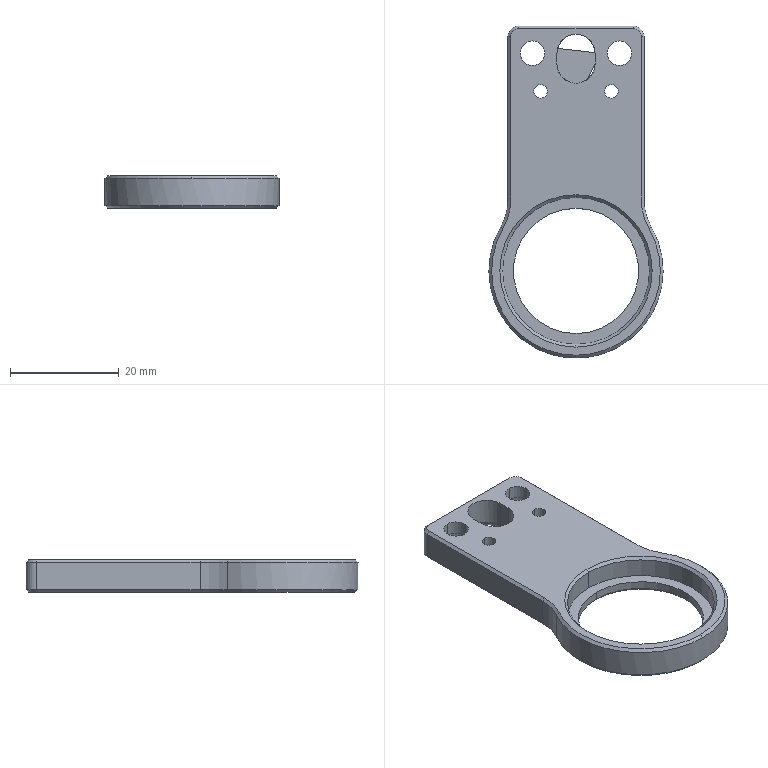NC program | NX | posted with a generic post | part box 32 x 61 x 6 mm
Lines 1418 to 2395 of 12533:
(ZLEVEL_PROFILE_1 , TOOL : D3R0.5)
N2816 T18 M6
N2818 G54
N2820 G17 G0 G90 X-13.711 Y2.712 S9500 M3
N2822 G43 Z30. H18
N2824 Z1.488
N2826 G94 G1 Z-0.012 F1000.
N2828 X-13.97 Y3.162
N2830 G3 X-14.23 Y3.312 R0.3
N2832 G1 X-23.46 F2500.
N2834 G3 X-25.864 Y2.367 R3.526
N2836 X-26.227 Y1.5 R1.142
N2838 G1 Y-1.5
N2840 G3 X-25.467 Y-2.711 R1.707
N2842 X-23.445 Y-3.312 R3.7
N2844 G1 X-5.
N2846 G3 X-1.688 Y0. R3.312
N2848 X-5. Y3.312 R3.312
N2850 G1 X-14.23
N2852 X-15.384 Y3.31
N2854 X-16.538 Y3.307
N2856 X-17.691 Y3.304 Z-0.013
N2858 X-18.845 Y3.302
N2860 X-19.999 Y3.299 Z-0.014
N2862 X-21.153 Y3.296
N2864 X-22.28 Y3.294
N2866 X-23.46 Y3.295 Z-0.015
N2868 X-23.98 Y3.228
N2870 X-24.486 Y3.104
N2872 X-24.977 Y2.928
N2874 X-25.437 Y2.676
N2876 X-25.832 Y2.346
N2878 X-25.989 Y2.165
N2880 X-26.107 Y1.954 Z-0.016
N2882 X-26.186 Y1.728
N2884 X-26.205 Y1.629
N2886 X-26.203 Y1.5
N2888 X-26.196 Y0.75
N2890 X-26.195 Y0.
N2892 X-26.193 Y-0.75
N2894 X-26.192 Y-1.5 Z-0.017
N2896 X-26.182 Y-1.682
N2898 X-26.11 Y-1.845
N2900 X-26.032 Y-2.008
N2902 X-25.947 Y-2.167
N2904 X-25.843 Y-2.3
N2906 X-25.713 Y-2.439
N2908 X-25.503 Y-2.604
N2910 X-25.428 Y-2.656
N2912 X-25.201 Y-2.793
N2914 X-24.97 Y-2.91
N2916 X-24.728 Y-3.014
N2918 X-24.48 Y-3.098
N2920 X-24.226 Y-3.165
N2922 X-23.969 Y-3.215 Z-0.018
N2924 X-23.486 Y-3.265
N2926 X-23.445 Y-3.267
N2928 X-22.127 Y-3.268
N2930 X-20.81 Y-3.265 Z-0.019
N2932 X-19.492 Y-3.263
N2934 X-18.175 Y-3.26
N2936 X-16.857 Y-3.258 Z-0.02
N2938 X-15.54 Y-3.255
N2940 X-14.222 Y-3.253 Z-0.021
N2942 X-12.905 Y-3.25
N2944 X-11.587 Y-3.248
N2946 X-10.27 Y-3.246 Z-0.022
N2948 X-8.952 Y-3.243
N2950 X-7.635 Y-3.241 Z-0.023
N2952 X-6.317 Y-3.239
N2954 X-5. Y-3.236
N2956 X-4.769 Y-3.228
N2958 X-4.54 Y-3.203
N2960 X-4.313 Y-3.161 Z-0.024
N2962 X-4.089 Y-3.104
N2964 X-3.87 Y-3.031
N2966 X-3.657 Y-2.942
N2968 X-3.451 Y-2.839
N2970 X-3.253 Y-2.721
N2972 X-3.064 Y-2.589
N2974 X-2.884 Y-2.444
N2976 X-2.716 Y-2.287
N2978 X-2.559 Y-2.118
N2980 X-2.415 Y-1.938
N2982 X-2.283 Y-1.749
N2984 X-2.166 Y-1.55
N2986 X-2.063 Y-1.344
N2988 X-1.975 Y-1.131 Z-0.025
N2990 X-1.902 Y-0.913
N2992 X-1.845 Y-0.69
N2994 X-1.805 Y-0.463
N2996 X-1.78 Y-0.234
N2998 X-1.772 Y-0.004
N3000 X-1.781 Y0.227
N3002 X-1.805 Y0.456
N3004 X-1.846 Y0.683
N3006 X-1.904 Y0.906
N3008 X-1.976 Y1.125
N3010 X-2.065 Y1.337
N3012 X-2.168 Y1.543
N3014 X-2.286 Y1.741
N3016 X-2.417 Y1.931 Z-0.026
N3018 X-2.562 Y2.11
N3020 X-2.719 Y2.278
N3022 X-2.888 Y2.435
N3024 X-3.067 Y2.579
N3026 X-3.257 Y2.71
N3028 X-3.455 Y2.827
N3030 X-3.661 Y2.93
N3032 X-3.873 Y3.018
N3034 X-4.092 Y3.09
N3036 X-4.315 Y3.147
N3038 X-4.541 Y3.187
N3040 X-4.77 Y3.212
N3042 X-5. Y3.22
N3044 X-6.154 Y3.218 Z-0.027
N3046 X-7.308 Y3.216
N3048 X-8.461 Y3.214 Z-0.028
N3050 X-9.615 Y3.212
N3052 X-10.769 Y3.21
N3054 X-11.923 Y3.209 Z-0.029
N3056 X-13.076 Y3.207
N3058 X-14.23 Y3.205
N3060 X-15.377 Y3.203 Z-0.03
N3062 X-16.524 Y3.2
N3064 X-17.671 Y3.198 Z-0.031
N3066 X-18.818 Y3.196
N3068 X-19.965 Y3.193 Z-0.032
N3070 X-21.112 Y3.191
N3072 X-22.259 Y3.189 Z-0.033
N3074 X-23.406
N3076 X-23.917 Y3.15
N3078 X-24.417 Y3.035 Z-0.034
N3080 X-24.895 Y2.851
N3082 X-25.34 Y2.597
N3084 X-25.629 Y2.379
N3086 X-25.735 Y2.276
N3088 X-25.89 Y2.073
N3090 X-26.012 Y1.869
N3092 X-26.108 Y1.618
N3094 X-26.097 Y1.5 Z-0.035
N3096 X-26.093 Y0.75
N3098 X-26.091 Y0.
N3100 X-26.09 Y-0.75
N3102 X-26.088 Y-1.5 Z-0.036
N3104 X-26.082 Y-1.666
N3106 X-26.02 Y-1.799
N3108 X-25.953 Y-1.94
N3110 X-25.876 Y-2.078
N3112 X-25.787 Y-2.195
N3114 X-25.677 Y-2.317
N3116 X-25.424 Y-2.533
N3118 X-25.087 Y-2.742
N3120 X-24.708 Y-2.918 Z-0.037
N3122 X-24.308 Y-3.041
N3124 X-23.9 Y-3.125
N3126 X-23.484 Y-3.171
N3128 X-23.348
N3130 X-22.096 Y-3.166 Z-0.038
N3132 X-20.844 Y-3.163
N3134 X-19.524 Y-3.161 Z-0.039
N3136 X-18.204 Y-3.158
N3138 X-16.883 Y-3.156 Z-0.04
N3140 X-15.563 Y-3.154
N3142 X-14.243 Y-3.151 Z-0.041
N3144 X-12.922 Y-3.149 Z-0.042
N3146 X-11.602 Y-3.147
N3148 X-10.281 Y-3.145 Z-0.043
N3150 X-8.961 Y-3.142
N3152 X-7.641 Y-3.14 Z-0.044
N3154 X-6.32 Y-3.138
N3156 X-5. Y-3.136 Z-0.045
N3158 X-4.754 Y-3.126
N3160 X-4.51 Y-3.096
N3162 X-4.269 Y-3.048
N3164 X-4.033 Y-2.981
N3166 X-3.802 Y-2.896
N3168 X-3.579 Y-2.792 Z-0.046
N3170 X-3.365 Y-2.672
N3172 X-3.161 Y-2.535
N3174 X-2.968 Y-2.383
N3176 X-2.787 Y-2.216
N3178 X-2.621 Y-2.036
N3180 X-2.469 Y-1.843
N3182 X-2.333 Y-1.639
N3184 X-2.213 Y-1.424
N3186 X-2.11 Y-1.201
N3188 X-2.025 Y-0.971 Z-0.047
N3190 X-1.959 Y-0.735
N3192 X-1.911 Y-0.494
N3194 X-1.882 Y-0.25
N3196 X-1.872 Y-0.005
N3198 X-1.882 Y0.24
N3200 X-1.911 Y0.484
N3202 X-1.959 Y0.725
N3204 X-2.026 Y0.962
N3206 X-2.111 Y1.192
N3208 X-2.214 Y1.416 Z-0.048
N3210 X-2.334 Y1.63
N3212 X-2.47 Y1.834
N3214 X-2.623 Y2.027
N3216 X-2.789 Y2.207
N3218 X-2.97 Y2.373
N3220 X-3.163 Y2.525
N3222 X-3.367 Y2.661
N3224 X-3.581 Y2.781
N3226 X-3.804 Y2.884 Z-0.049
N3228 X-4.034 Y2.968
N3230 X-4.271 Y3.034
N3232 X-4.511 Y3.082
N3234 X-4.755 Y3.11
N3236 X-5. Y3.12
N3238 X-6.154 Y3.118
N3240 X-7.308 Y3.116 Z-0.05
N3242 X-8.461 Y3.114
N3244 X-9.615 Y3.112 Z-0.051
N3246 X-10.769 Y3.111
N3248 X-11.923 Y3.109 Z-0.052
N3250 X-13.076 Y3.107
N3252 X-14.23 Y3.105 Z-0.053
N3254 X-15.374 Y3.103
N3256 X-16.519 Y3.101 Z-0.054
N3258 X-17.663 Y3.099 Z-0.055
N3260 X-18.807 Y3.096
N3262 X-19.952 Y3.094 Z-0.056
N3264 X-21.096 Y3.092 Z-0.057
N3266 X-22.206 Y3.09
N3268 X-23.315 Y3.089 Z-0.058
N3270 X-23.384
N3272 X-23.855 Y3.049
N3274 X-24.315 Y2.945
N3276 X-24.764 Y2.797 Z-0.059
N3278 X-25.183 Y2.579
N3280 X-25.487 Y2.372
N3282 X-25.568 Y2.307
N3284 X-25.73 Y2.137
N3286 X-25.809 Y2.026
N3288 X-25.863 Y1.944
N3290 X-25.899 Y1.876
N3292 X-25.917 Y1.842
N3294 X-25.933 Y1.806
N3296 X-25.952 Y1.728
N3298 X-25.999 Y1.5 Z-0.06
N3300 X-25.994 Y0.75
N3302 X-25.993 Y0.
N3304 X-25.992 Y-0.75 Z-0.061
N3306 X-25.993 Y-1.5
N3308 X-25.985 Y-1.591
N3310 X-25.968 Y-1.687
N3312 X-25.92 Y-1.783
N3314 X-25.856 Y-1.915
N3316 X-25.787 Y-2.045
N3318 X-25.715 Y-2.133 Z-0.062
N3320 X-25.595 Y-2.264
N3322 X-25.368 Y-2.455
N3324 X-25.14 Y-2.599
N3326 X-24.903 Y-2.72
N3328 X-24.654 Y-2.82
N3330 X-24.401 Y-2.903
N3332 X-24.143 Y-2.972 Z-0.063
N3334 X-23.881 Y-3.025
N3336 X-23.358 Y-3.073
N3338 X-22.042 Y-3.068 Z-0.064
N3340 X-20.727 Y-3.065
N3342 X-19.416 Y-3.063 Z-0.065
N3344 X-18.106 Y-3.061 Z-0.066
N3346 X-16.795 Y-3.058
N3348 X-15.485 Y-3.056 Z-0.067
N3350 X-14.174 Y-3.054 Z-0.068
N3352 X-12.863 Y-3.052 Z-0.069
N3354 X-11.553 Y-3.049
N3356 X-10.242 Y-3.047 Z-0.07
N3358 X-8.932 Y-3.045 Z-0.071
N3360 X-7.621 Y-3.043
N3362 X-6.311 Y-3.04 Z-0.072
N3364 X-5. Y-3.038 Z-0.073
N3366 X-4.762 Y-3.029
N3368 X-4.525 Y-3.
N3370 X-4.292 Y-2.953
N3372 X-4.062 Y-2.888
N3374 X-3.839 Y-2.806
N3376 X-3.623 Y-2.706 Z-0.074
N3378 X-3.415 Y-2.589
N3380 X-3.217 Y-2.456
N3382 X-3.03 Y-2.309
N3384 X-2.856 Y-2.147
N3386 X-2.694 Y-1.972
N3388 X-2.547 Y-1.785
N3390 X-2.415 Y-1.587
N3392 X-2.299 Y-1.379 Z-0.075
N3394 X-2.2 Y-1.163
N3396 X-2.117 Y-0.94
N3398 X-2.053 Y-0.711
N3400 X-2.007 Y-0.478
N3402 X-1.979 Y-0.241
N3404 X-1.97 Y-0.004
N3406 X-1.979 Y0.234 Z-0.076
N3408 X-2.007 Y0.471
N3410 X-2.054 Y0.704
N3412 X-2.118 Y0.933
N3414 X-2.201 Y1.156
N3416 X-2.301 Y1.372
N3418 X-2.417 Y1.58
N3420 X-2.549 Y1.778
N3422 X-2.697 Y1.964 Z-0.077
N3424 X-2.859 Y2.139
N3426 X-3.033 Y2.3
N3428 X-3.22 Y2.447
N3430 X-3.418 Y2.579
N3432 X-3.626 Y2.695
N3434 X-3.842 Y2.794
N3436 X-4.065 Y2.876
N3438 X-4.294 Y2.94 Z-0.078
N3440 X-4.527 Y2.986
N3442 X-4.763 Y3.014
N3444 X-5. Y3.023
N3446 X-6.154 Y3.021 Z-0.079
N3448 X-7.308 Y3.019
N3450 X-8.461 Y3.017 Z-0.08
N3452 X-9.615 Y3.015
N3454 X-10.769 Y3.014 Z-0.081
N3456 X-11.923 Y3.012 Z-0.082
N3458 X-13.076 Y3.01
N3460 X-14.23 Y3.008 Z-0.083
N3462 X-15.366 Y3.006 Z-0.084
N3464 X-16.501 Y3.004
N3466 X-17.637 Y3.002 Z-0.085
N3468 X-18.773 Y3. Z-0.086
N3470 X-19.908 Y2.998 Z-0.087
N3472 X-21.044 Y2.995
N3474 X-22.18 Y2.993 Z-0.088
N3476 X-23.315 Z-0.089
N3478 X-23.766 Y2.961
N3480 X-24.211 Y2.877
N3482 X-24.641 Y2.736 Z-0.09
N3484 X-25.049 Y2.542
N3486 X-25.309 Y2.383
N3488 X-25.425 Y2.294
N3490 X-25.495 Y2.23
N3492 X-25.602 Y2.131 Z-0.091
N3494 X-25.749 Y1.946
N3496 X-25.789 Y1.882
N3498 X-25.825 Y1.812
N3500 X-25.849 Y1.73
N3502 X-25.877 Y1.615
N3504 X-25.901 Y1.5
N3506 X-25.898 Y0.75
N3508 X-25.897 Y0. Z-0.092
N3510 X-25.896 Y-0.75
N3512 Y-1.5 Z-0.093
N3514 X-25.889 Y-1.596
N3516 X-25.87 Y-1.683
N3518 X-25.834 Y-1.762
N3520 X-25.704 Y-2.001
N3522 X-25.517 Y-2.197 Z-0.094
N3524 X-25.429 Y-2.277
N3526 X-25.142 Y-2.475
N3528 X-24.726 Y-2.691
N3530 X-24.282 Y-2.84
N3532 X-23.823 Y-2.929 Z-0.095
N3534 X-23.341 Y-2.973
N3536 X-22.038 Y-2.972 Z-0.096
N3538 X-20.735 Y-2.97 Z-0.097
N3540 X-19.424 Y-2.968 Z-0.098
N3542 X-18.113 Y-2.965 Z-0.099
N3544 X-16.801 Y-2.963
N3546 X-15.49 Y-2.961 Z-0.1
N3548 X-14.179 Y-2.959 Z-0.101
N3550 X-12.868 Y-2.956 Z-0.102
N3552 X-11.556 Y-2.954 Z-0.103
N3554 X-10.245 Y-2.952 Z-0.104
N3556 X-8.934 Y-2.95 Z-0.105
N3558 X-7.623 Y-2.948
N3560 X-6.311 Y-2.945 Z-0.106
N3562 X-5. Y-2.943 Z-0.107
N3564 X-4.769 Y-2.934
N3566 X-4.54 Y-2.906
N3568 X-4.314 Y-2.861 Z-0.108
N3570 X-4.092 Y-2.798
N3572 X-3.876 Y-2.718
N3574 X-3.666 Y-2.621
N3576 X-3.465 Y-2.508
N3578 X-3.273 Y-2.38
N3580 X-3.093 Y-2.237 Z-0.109
N3582 X-2.923 Y-2.08
N3584 X-2.767 Y-1.911
N3586 X-2.624 Y-1.73
N3588 X-2.496 Y-1.538
N3590 X-2.384 Y-1.337
N3592 X-2.288 Y-1.128
N3594 X-2.208 Y-0.912 Z-0.11
N3596 X-2.145 Y-0.69
N3598 X-2.1 Y-0.464
N3600 X-2.073 Y-0.235
N3602 X-2.064 Y-0.005
N3604 X-2.073 Y0.225
N3606 X-2.1 Y0.454
N3608 X-2.145 Y0.681 Z-0.111
N3610 X-2.208 Y0.903
N3612 X-2.288 Y1.119
N3614 X-2.385 Y1.329
N3616 X-2.497 Y1.53
N3618 X-2.626 Y1.721
N3620 X-2.768 Y1.902 Z-0.112
N3622 X-2.925 Y2.071
N3624 X-3.094 Y2.228
N3626 X-3.275 Y2.37
N3628 X-3.467 Y2.498
N3630 X-3.668 Y2.61
N3632 X-3.877 Y2.707
N3634 X-4.094 Y2.786 Z-0.113
N3636 X-4.315 Y2.848
N3638 X-4.541 Y2.893
N3640 X-4.77 Y2.92
N3642 X-5. Y2.928
N3644 X-6.154 Y2.926 Z-0.114
N3646 X-7.308 Y2.925 Z-0.115
N3648 X-8.461 Y2.923
N3650 X-9.615 Y2.921 Z-0.116
N3652 X-10.769 Y2.919 Z-0.117
N3654 X-11.923 Y2.917 Z-0.118
N3656 X-13.076 Y2.916 Z-0.119
N3658 X-14.23 Y2.914
N3660 X-15.364 Y2.912 Z-0.12
N3662 X-16.499 Y2.91 Z-0.121
N3664 X-17.633 Y2.908 Z-0.122
N3666 X-18.767 Y2.906 Z-0.123
N3668 X-19.901 Y2.903 Z-0.124
N3670 X-21.036 Y2.901 Z-0.125
N3672 X-22.17 Y2.899
N3674 X-23.304 Z-0.126
N3676 X-23.819 Y2.852 Z-0.127
N3678 X-24.072 Y2.799
N3680 X-24.325 Y2.746
N3682 X-24.807 Y2.56 Z-0.128
N3684 X-25.056 Y2.433
N3686 X-25.258 Y2.305
N3688 X-25.358 Y2.223
N3690 X-25.5 Y2.101
N3692 X-25.648 Y1.925
N3694 X-25.716 Y1.81 Z-0.129
N3696 X-25.758 Y1.723
N3698 X-25.785 Y1.653
N3700 X-25.801 Y1.578
N3702 X-25.808 Y1.5
N3704 X-25.805 Y0.75
N3706 X-25.804 Y0. Z-0.13
N3708 X-25.802 Y-0.75 Z-0.131
N3710 X-25.803 Y-1.5
N3712 X-25.794 Y-1.594
N3714 X-25.785 Y-1.639
N3716 X-25.77 Y-1.684
N3718 X-25.725 Y-1.768
N3720 X-25.574 Y-2.007 Z-0.132
N3722 X-25.505 Y-2.08
N3724 X-25.374 Y-2.206
N3726 X-25.341 Y-2.231
N3728 X-25.011 Y-2.445
N3730 X-24.616 Y-2.631
N3732 X-24.202 Y-2.764 Z-0.133
N3734 X-23.775 Y-2.851
N3736 X-23.558 Y-2.866
N3738 X-23.286 Y-2.883 Z-0.134
N3740 X-22.003 Y-2.879 Z-0.135
N3742 X-20.721 Y-2.877 Z-0.136
N3744 X-19.411 Y-2.875 Z-0.137
N3746 X-18.101 Y-2.873 Z-0.138
N3748 X-16.791 Y-2.87 Z-0.139
N3750 X-15.481 Y-2.868 Z-0.14
N3752 X-14.171 Y-2.866 Z-0.141
N3754 X-12.861 Y-2.864 Z-0.142
N3756 X-11.55 Y-2.862 Z-0.143
N3758 X-10.24 Y-2.859 Z-0.144
N3760 X-8.93 Y-2.857 Z-0.145
N3762 X-7.62 Y-2.855 Z-0.146
N3764 X-6.31 Y-2.853 Z-0.147
N3766 X-5. Y-2.851 Z-0.148
N3768 X-4.776 Y-2.842
N3770 X-4.554 Y-2.815
N3772 X-4.335 Y-2.771
N3774 X-4.12 Y-2.71
N3776 X-3.91 Y-2.632 Z-0.149
N3778 X-3.707 Y-2.538
N3780 X-3.512 Y-2.429
N3782 X-3.327 Y-2.305
N3784 X-3.151 Y-2.166
N3786 X-2.988 Y-2.014 Z-0.15
N3788 X-2.836 Y-1.85
N3790 X-2.698 Y-1.674
N3792 X-2.574 Y-1.488
N3794 X-2.465 Y-1.293
N3796 X-2.372 Y-1.09
N3798 X-2.295 Y-0.881 Z-0.151
N3800 X-2.234 Y-0.666
N3802 X-2.191 Y-0.447
N3804 X-2.165 Y-0.225
N3806 X-2.156 Y-0.002
N3808 X-2.165 Y0.221
N3810 X-2.192 Y0.443 Z-0.152
N3812 X-2.236 Y0.662
N3814 X-2.296 Y0.877
N3816 X-2.374 Y1.086
N3818 X-2.468 Y1.289
N3820 X-2.577 Y1.483
N3822 X-2.701 Y1.669 Z-0.153
N3824 X-2.839 Y1.844
N3826 X-2.991 Y2.007
N3828 X-3.155 Y2.159
N3830 X-3.33 Y2.297
N3832 X-3.516 Y2.42 Z-0.154
N3834 X-3.711 Y2.529
N3836 X-3.913 Y2.622
N3838 X-4.123 Y2.699
N3840 X-4.337 Y2.759
N3842 X-4.556 Y2.802
N3844 X-4.777 Y2.828 Z-0.155
N3846 X-5. Y2.837
N3848 X-6.154 Y2.835 Z-0.156
N3850 X-7.308 Y2.833 Z-0.157
N3852 X-8.461 Y2.831
N3854 X-9.615 Y2.829 Z-0.158
N3856 X-10.769 Y2.827 Z-0.159
N3858 X-11.923 Y2.826 Z-0.16
N3860 X-13.076 Y2.824 Z-0.161
N3862 X-14.23 Y2.822 Z-0.162
N3864 X-15.364 Y2.82 Z-0.163
N3866 X-16.498 Y2.818 Z-0.164
N3868 X-17.631 Y2.816 Z-0.165
N3870 X-18.765 Y2.814 Z-0.166
N3872 X-19.899 Y2.812 Z-0.167
N3874 X-21.032 Y2.81 Z-0.168
N3876 X-22.166 Y2.808 Z-0.169
N3878 X-23.333 Y2.806 Z-0.17
N3880 X-23.726 Y2.773
N3882 X-24.147 Y2.694 Z-0.171
N3884 X-24.556 Y2.569
N3886 X-24.75 Y2.478
N3888 X-24.943 Y2.388 Z-0.172
N3890 X-25.115 Y2.278
N3892 X-25.285 Y2.167
N3894 X-25.31 Y2.147
N3896 X-25.496 Y1.971
N3898 X-25.552 Y1.907
N3900 X-25.6 Y1.829
N3902 X-25.643 Y1.752
N3904 X-25.688 Y1.634 Z-0.173
N3906 X-25.71 Y1.555
N3908 X-25.717 Y1.5
N3910 X-25.714 Y0.75
N3912 X-25.713 Y0. Z-0.174
N3914 X-25.712 Y-0.75 Z-0.175
N3916 X-25.711 Y-1.5
N3918 X-25.699 Y-1.59
N3920 X-25.69 Y-1.634 Z-0.176
N3922 X-25.675 Y-1.675
N3924 X-25.634 Y-1.753
N3926 X-25.578 Y-1.853
N3928 X-25.546 Y-1.899
N3930 X-25.482 Y-1.974
N3932 X-25.323 Y-2.125
N3934 X-25.286 Y-2.154
N3936 X-25.108 Y-2.272
N3938 X-24.927 Y-2.386
N3940 X-24.733 Y-2.475 Z-0.177
N3942 X-24.539 Y-2.563
N3944 X-24.129 Y-2.682
N3946 X-23.711 Y-2.759 Z-0.178
N3948 X-23.515 Y-2.774
N3950 X-23.286 Y-2.791
N3952 X-21.98 Y-2.789 Z-0.179
N3954 X-20.673 Y-2.787 Z-0.18
N3956 X-19.367 Y-2.785 Z-0.182
N3958 X-18.061 Y-2.783 Z-0.183
N3960 X-16.755 Y-2.78 Z-0.184
N3962 X-15.449 Y-2.778 Z-0.185
N3964 X-14.143 Y-2.776 Z-0.186
N3966 X-12.837 Y-2.774 Z-0.187
N3968 X-11.531 Y-2.772 Z-0.189
N3970 X-10.224 Y-2.77 Z-0.19
N3972 X-8.918 Y-2.768 Z-0.191
N3974 X-7.612 Y-2.766 Z-0.192
N3976 X-6.306 Y-2.764 Z-0.193
N3978 X-5. Y-2.761 Z-0.194
N3980 X-4.784 Y-2.753 Z-0.195
N3982 X-4.568 Y-2.727
N3984 X-4.356 Y-2.684
N3986 X-4.148 Y-2.625
N3988 X-3.945 Y-2.55
N3990 X-3.748 Y-2.459 Z-0.196
N3992 X-3.56 Y-2.353
N3994 X-3.38 Y-2.233
N3996 X-3.21 Y-2.099
N3998 X-3.051 Y-1.952
N4000 X-2.904 Y-1.793 Z-0.197
N4002 X-2.771 Y-1.623
N4004 X-2.651 Y-1.443
N4006 X-2.545 Y-1.254
N4008 X-2.455 Y-1.057
N4010 X-2.38 Y-0.854 Z-0.198
N4012 X-2.321 Y-0.646
N4014 X-2.279 Y-0.434
N4016 X-2.254 Y-0.22
N4018 X-2.245 Y-0.004
N4020 X-2.254 Y0.213
N4022 X-2.279 Y0.427 Z-0.199
N4024 X-2.322 Y0.64
N4026 X-2.381 Y0.848
N4028 X-2.456 Y1.051
N4030 X-2.546 Y1.247
N4032 X-2.652 Y1.436 Z-0.2
N4034 X-2.772 Y1.616
N4036 X-2.906 Y1.785
N4038 X-3.053 Y1.944
N4040 X-3.212 Y2.091
N4042 X-3.382 Y2.224 Z-0.201
N4044 X-3.562 Y2.344
N4046 X-3.751 Y2.45
N4048 X-3.947 Y2.54
N4050 X-4.15 Y2.614
N4052 X-4.358 Y2.673 Z-0.202
N4054 X-4.57 Y2.715
N4056 X-4.784 Y2.74
N4058 X-5. Y2.748
N4060 X-6.154 Y2.746 Z-0.203
N4062 X-7.308 Y2.744 Z-0.204
N4064 X-8.461 Y2.743 Z-0.205
N4066 X-9.615 Y2.741 Z-0.206
N4068 X-10.769 Y2.739 Z-0.207
N4070 X-11.923 Y2.737 Z-0.208
N4072 X-13.076 Y2.736 Z-0.209
N4074 X-14.23 Y2.734 Z-0.21
N4076 X-15.368 Y2.732 Z-0.212
N4078 X-16.506 Y2.73 Z-0.213
N4080 X-17.643 Y2.728 Z-0.214
N4082 X-18.781 Y2.726 Z-0.215
N4084 X-19.919 Y2.724 Z-0.216
N4086 X-21.057 Y2.722 Z-0.217
N4088 X-22.17 Y2.72 Z-0.219
N4090 X-23.332 Y2.717 Z-0.22
N4092 X-23.737 Y2.683
N4094 X-24.136 Y2.609 Z-0.221
N4096 X-24.524 Y2.488
N4098 X-24.892 Y2.314
N4100 X-25.141 Y2.161 Z-0.222
N4102 X-25.257 Y2.076
N4104 X-25.31 Y2.026
N4106 X-25.477 Y1.855
N4108 X-25.544 Y1.752
N4110 X-25.583 Y1.689
N4112 X-25.611 Y1.609
N4114 X-25.629 Y1.5
N4116 X-25.627 Y0.75 Z-0.223
N4118 X-25.626 Y0. Z-0.224
N4120 X-25.624 Y-0.75 Z-0.225
N4122 Y-1.5 Z-0.226
N4124 X-25.615 Y-1.575
N4126 X-25.606 Y-1.611
N4128 X-25.594 Y-1.646
N4130 X-25.558 Y-1.713
N4132 X-25.43 Y-1.898
N4134 X-25.301 Y-2.032
N4136 X-25.272 Y-2.059
N4138 X-25.098 Y-2.175
N4140 X-24.923 Y-2.289 Z-0.227
N4142 X-24.545 Y-2.47
N4144 X-24.145 Y-2.593
N4146 X-23.735 Y-2.67 Z-0.228
N4148 X-23.319 Y-2.701
N4150 X-22.01 Y-2.702 Z-0.23
N4152 X-20.702 Y-2.7 Z-0.231
N4154 X-19.393 Y-2.698 Z-0.232
N4156 X-18.085 Y-2.696 Z-0.234
N4158 X-16.776 Y-2.694 Z-0.235
N4160 X-15.468 Y-2.692 Z-0.236
N4162 X-14.159 Y-2.69 Z-0.238
N4164 X-12.851 Y-2.688 Z-0.239
N4166 X-11.542 Y-2.686 Z-0.24
N4168 X-10.234 Y-2.684 Z-0.242
N4170 X-8.925 Y-2.682 Z-0.243
N4172 X-7.617 Y-2.68 Z-0.244
N4174 X-6.308 Y-2.678 Z-0.246
N4176 X-5. Y-2.676 Z-0.247
N4178 X-4.79 Y-2.667
N4180 X-4.582 Y-2.642
N4182 X-4.376 Y-2.601 Z-0.248
N4184 X-4.175 Y-2.544
N4186 X-3.978 Y-2.471
N4188 X-3.788 Y-2.383
N4190 X-3.605 Y-2.28
N4192 X-3.431 Y-2.164 Z-0.249
N4194 X-3.266 Y-2.034
N4196 X-3.112 Y-1.891
N4198 X-2.97 Y-1.738
N4200 X-2.84 Y-1.573
N4202 X-2.724 Y-1.399 Z-0.25
N4204 X-2.622 Y-1.216
N4206 X-2.534 Y-1.026
N4208 X-2.462 Y-0.829
N4210 X-2.405 Y-0.628
N4212 X-2.364 Y-0.422 Z-0.251
N4214 X-2.339 Y-0.214
N4216 X-2.331 Y-0.005
N4218 X-2.339 Y0.204
N4220 X-2.364 Y0.413 Z-0.252
N4222 X-2.404 Y0.619
N4224 X-2.461 Y0.82
N4226 X-2.534 Y1.017
N4228 X-2.622 Y1.208
N4230 X-2.724 Y1.391 Z-0.253
N4232 X-2.841 Y1.565
N4234 X-2.971 Y1.729
N4236 X-3.113 Y1.883
N4238 X-3.267 Y2.025
N4240 X-3.432 Y2.155 Z-0.254
N4242 X-3.606 Y2.271
N4244 X-3.789 Y2.374
N4246 X-3.979 Y2.461
N4248 X-4.176 Y2.533 Z-0.255
N4250 X-4.377 Y2.59
N4252 X-4.583 Y2.631
N4254 X-4.791 Y2.655
N4256 X-5. Y2.663
N4258 X-6.154 Y2.661 Z-0.257
N4260 X-7.308 Y2.659 Z-0.258
N4262 X-8.461 Y2.658 Z-0.259
N4264 X-9.615 Y2.656 Z-0.26
N4266 X-10.769 Y2.654 Z-0.261
N4268 X-11.923 Y2.652 Z-0.262
N4270 X-13.076 Y2.651 Z-0.264
N4272 X-14.23 Y2.649 Z-0.265
N4274 X-15.362 Y2.647 Z-0.266
N4276 X-16.494 Y2.645 Z-0.267
N4278 X-17.625 Y2.644 Z-0.269
N4280 X-18.757 Y2.642 Z-0.27
N4282 X-19.889 Y2.64 Z-0.271
N4284 X-21.02 Y2.638 Z-0.272
N4286 X-22.096 Y2.636 Z-0.274
N4288 X-23.172 Y2.635 Z-0.275
N4290 X-23.283
N4292 X-23.761 Y2.594
N4294 X-23.995 Y2.546 Z-0.276
N4296 X-24.229 Y2.495
N4298 X-24.678 Y2.328 Z-0.277
N4300 X-24.804 Y2.267
N4302 X-24.95 Y2.182
N4304 X-25.096 Y2.096
N4306 X-25.255 Y1.969
N4308 X-25.387 Y1.833 Z-0.278
N4310 X-25.439 Y1.762
N4312 X-25.492 Y1.675
N4314 X-25.506 Y1.644
N4316 X-25.537 Y1.555
N4318 X-25.545 Y1.5
N4320 X-25.543 Y0.75 Z-0.279
N4322 X-25.542 Y0. Z-0.28
N4324 X-25.541 Y-0.75
N4326 Y-1.5 Z-0.281
N4328 X-25.533 Y-1.555
N4330 X-25.527 Y-1.582
N4332 X-25.515 Y-1.614
N4334 X-25.483 Y-1.675 Z-0.282
N4336 X-25.378 Y-1.833
N4338 X-25.331 Y-1.884
N4340 X-25.245 Y-1.967
N4342 X-25.091 Y-2.089
N4344 X-24.908 Y-2.201
N4346 X-24.724 Y-2.295 Z-0.283
N4348 X-24.536 Y-2.382
N4350 X-24.142 Y-2.506
N4352 X-23.737 Y-2.59 Z-0.284
N4354 X-23.325 Y-2.619
N4356 X-23.26 Y-2.621
N4358 X-21.984 Y-2.619 Z-0.286
N4360 X-20.708 Y-2.617 Z-0.287
N4362 X-19.399 Y-2.615 Z-0.289
N4364 X-18.09 Y-2.613 Z-0.29
N4366 X-16.781 Y-2.611 Z-0.292
N4368 X-15.472 Y-2.609 Z-0.293
N4370 X-14.163 Y-2.607 Z-0.295
N4372 X-12.854 Y-2.605 Z-0.296
N4374 X-11.545 Y-2.603 Z-0.298
N4376 X-10.236 Y-2.601 Z-0.299
N4378 X-8.927 Y-2.599 Z-0.3
N4380 X-7.618 Y-2.597 Z-0.302
N4382 X-6.309 Y-2.595 Z-0.303
N4384 X-5. Y-2.594 Z-0.305
N4386 X-4.797 Y-2.585
N4388 X-4.595 Y-2.561
N4390 X-4.395 Y-2.521 Z-0.306
N4392 X-4.199 Y-2.466
N4394 X-4.009 Y-2.395
N4396 X-3.824 Y-2.31
N4398 X-3.647 Y-2.21
N4400 X-3.478 Y-2.097 Z-0.307
N4402 X-3.318 Y-1.971
N4404 X-3.169 Y-1.833
N4406 X-3.031 Y-1.683
N4408 X-2.906 Y-1.523 Z-0.308
N4410 X-2.793 Y-1.354
N4412 X-2.694 Y-1.177
N4414 X-2.609 Y-0.992
N4416 X-2.539 Y-0.802 Z-0.309
N4418 X-2.484 Y-0.606
N4420 X-2.444 Y-0.407
N4422 X-2.42 Y-0.205
N4424 X-2.412 Y-0.002
N4426 X-2.421 Y0.201 Z-0.31
N4428 X-2.445 Y0.403
N4430 X-2.484 Y0.602
N4432 X-2.54 Y0.797
N4434 X-2.61 Y0.988 Z-0.311
N4436 X-2.695 Y1.172
N4438 X-2.795 Y1.35
N4440 X-2.908 Y1.518
N4442 X-3.034 Y1.678 Z-0.312
N4444 X-3.172 Y1.827
N4446 X-3.321 Y1.964
N4448 X-3.48 Y2.09
N4450 X-3.649 Y2.202
N4452 X-3.827 Y2.301 Z-0.313
N4454 X-4.011 Y2.386
N4456 X-4.201 Y2.456
N4458 X-4.397 Y2.511
N4460 X-4.596 Y2.55 Z-0.314
N4462 X-4.797 Y2.574
N4464 X-5. Y2.582
N4466 X-6.154 Y2.58 Z-0.315
N4468 X-7.308 Y2.578 Z-0.317
N4470 X-8.461 Y2.577 Z-0.318
N4472 X-9.615 Y2.575 Z-0.319
N4474 X-10.769 Y2.573 Z-0.321
N4476 X-11.923 Y2.572 Z-0.322
N4478 X-13.076 Y2.57 Z-0.323
N4480 X-14.23 Y2.568 Z-0.324
N4482 X-15.72 Y2.566 Z-0.326
N4484 X-17.211 Y2.564 Z-0.328
N4486 X-18.701 Y2.562 Z-0.33
N4488 X-20.191 Y2.559 Z-0.332
N4490 X-21.681 Y2.557 Z-0.333
N4492 X-23.172 Y2.555 Z-0.335
N4494 X-23.584 Y2.534 Z-0.336
N4496 X-23.992 Y2.469
N4498 X-24.39 Y2.358 Z-0.337
N4500 X-24.58 Y2.279
N4502 X-24.769 Y2.198
N4504 X-24.807 Y2.178
N4506 X-25.028 Y2.047 Z-0.338
N4508 X-25.134 Y1.965
N4510 X-25.255 Y1.851
N4512 X-25.347 Y1.746
N4514 X-25.415 Y1.651
N4516 X-25.436 Y1.616
N4518 X-25.453 Y1.563
N4520 X-25.465 Y1.5 Z-0.339
N4522 X-25.464 Y0.75
N4524 X-25.463 Y0. Z-0.34
N4526 X-25.462 Y-0.75 Z-0.341
N4528 X-25.461 Y-1.5 Z-0.342
N4530 X-25.455 Y-1.545
N4532 X-25.431 Y-1.608
N4534 X-25.372 Y-1.704
N4536 X-25.294 Y-1.804 Z-0.343
N4538 X-25.224 Y-1.879
N4540 X-25.049 Y-2.025
N4542 X-25.02 Y-2.043
N4544 X-24.829 Y-2.149
N4546 X-24.635 Y-2.252 Z-0.344
N4548 X-24.415 Y-2.336
N4550 X-24.192 Y-2.413
N4552 X-23.73 Y-2.505 Z-0.345
N4554 X-23.272 Y-2.541
N4556 X-21.962 Z-0.347
N4558 X-20.652 Y-2.539 Z-0.349
N4560 X-19.347 Y-2.537 Z-0.35
N4562 X-18.043 Y-2.535 Z-0.352
N4564 X-16.739 Y-2.533 Z-0.353
N4566 X-15.434 Y-2.531 Z-0.355
N4568 X-14.13 Y-2.529 Z-0.356
N4570 X-12.826 Y-2.527 Z-0.358
N4572 X-11.522 Y-2.526 Z-0.36
N4574 X-10.217 Y-2.524 Z-0.361
N4576 X-8.913 Y-2.522 Z-0.363
N4578 X-7.609 Y-2.52 Z-0.364
N4580 X-6.304 Y-2.518 Z-0.366
N4582 X-5. Y-2.516 Z-0.368
N4584 X-4.781 Y-2.506
N4586 X-4.564 Y-2.478
N4588 X-4.35 Y-2.43
N4590 X-4.141 Y-2.364 Z-0.369
N4592 X-3.938 Y-2.28
N4594 X-3.744 Y-2.178
N4596 X-3.559 Y-2.06
N4598 X-3.385 Y-1.927 Z-0.37
N4600 X-3.224 Y-1.779
N4602 X-3.076 Y-1.617
N4604 X-2.943 Y-1.443 Z-0.371
N4606 X-2.825 Y-1.259
N4608 X-2.724 Y-1.064
N4610 X-2.64 Y-0.862
N4612 X-2.575 Y-0.653 Z-0.372
N4614 X-2.527 Y-0.439
N4616 X-2.499 Y-0.223
N4618 X-2.489 Y-0.004
N4620 X-2.499 Y0.215 Z-0.373
N4622 X-2.527 Y0.433
N4624 X-2.575 Y0.647
N4626 X-2.641 Y0.856
N4628 X-2.725 Y1.058 Z-0.374
N4630 X-2.826 Y1.252
N4632 X-2.944 Y1.437
N4634 X-3.077 Y1.611
N4636 X-3.225 Y1.772 Z-0.375
N4638 X-3.387 Y1.92
N4640 X-3.561 Y2.053
N4642 X-3.745 Y2.171 Z-0.376
N4644 X-3.94 Y2.272
N4646 X-4.142 Y2.355
N4648 X-4.351 Y2.421
N4650 X-4.564 Y2.468 Z-0.377
N4652 X-4.781 Y2.496
N4654 X-5. Y2.505
N4656 X-6.154 Y2.504 Z-0.379
N4658 X-7.308 Y2.502 Z-0.38
N4660 X-8.461 Y2.501 Z-0.381
N4662 X-9.615 Y2.499 Z-0.383
N4664 X-10.769 Y2.498 Z-0.384
N4666 X-11.923 Y2.496 Z-0.386
N4668 X-13.076 Y2.494 Z-0.387
N4670 X-14.23 Y2.493 Z-0.388
N4672 X-15.72 Y2.491 Z-0.39
N4674 X-17.211 Y2.489 Z-0.392
N4676 X-18.701 Y2.486 Z-0.394
N4678 X-20.191 Y2.484 Z-0.396
N4680 X-21.681 Y2.482 Z-0.398
N4682 X-23.172 Y2.481 Z-0.4
N4684 X-23.586 Y2.46 Z-0.401
N4686 X-23.995 Y2.393
N4688 X-24.194 Y2.338
N4690 X-24.392 Y2.276 Z-0.402
N4692 X-24.583 Y2.195
N4694 X-24.773 Y2.113
N4696 X-24.805 Y2.097
N4698 X-25.055 Y1.932 Z-0.403
N4700 X-25.182 Y1.825
N4702 X-25.293 Y1.704
N4704 X-25.355 Y1.605
N4706 X-25.383 Y1.543
N4708 X-25.392 Y1.5
N4710 X-25.39 Y0.75 Z-0.404
N4712 X-25.389 Y0. Z-0.405
N4714 X-25.388 Y-0.76 Z-0.406
N4716 X-25.386 Y-1.52 Z-0.407
N4718 X-25.362 Y-1.582
N4720 X-25.293 Y-1.691 Z-0.408
N4722 X-25.239 Y-1.757
N4724 X-25.162 Y-1.835
N4726 X-25.094 Y-1.891
N4728 X-24.981 Y-1.98
N4730 X-24.786 Y-2.091
N4732 X-24.584 Y-2.192 Z-0.409
N4734 X-24.373 Y-2.27
N4736 X-24.161 Y-2.344
N4738 X-23.941 Y-2.391 Z-0.41
N4740 X-23.72 Y-2.434
N4742 X-23.254 Y-2.468
N4744 X-21.957 Y-2.467 Z-0.412
N4746 X-20.661 Y-2.465 Z-0.414
N4748 X-19.356 Y-2.464 Z-0.416
N4750 X-18.051 Y-2.462 Z-0.417
N4752 X-16.746 Y-2.46 Z-0.419
N4754 X-15.441 Y-2.458 Z-0.421
N4756 X-14.136 Y-2.457 Z-0.422
N4758 X-12.831 Y-2.455 Z-0.424
N4760 X-11.526 Y-2.453 Z-0.426
N4762 X-10.22 Y-2.451 Z-0.427
N4764 X-8.915 Y-2.45 Z-0.429